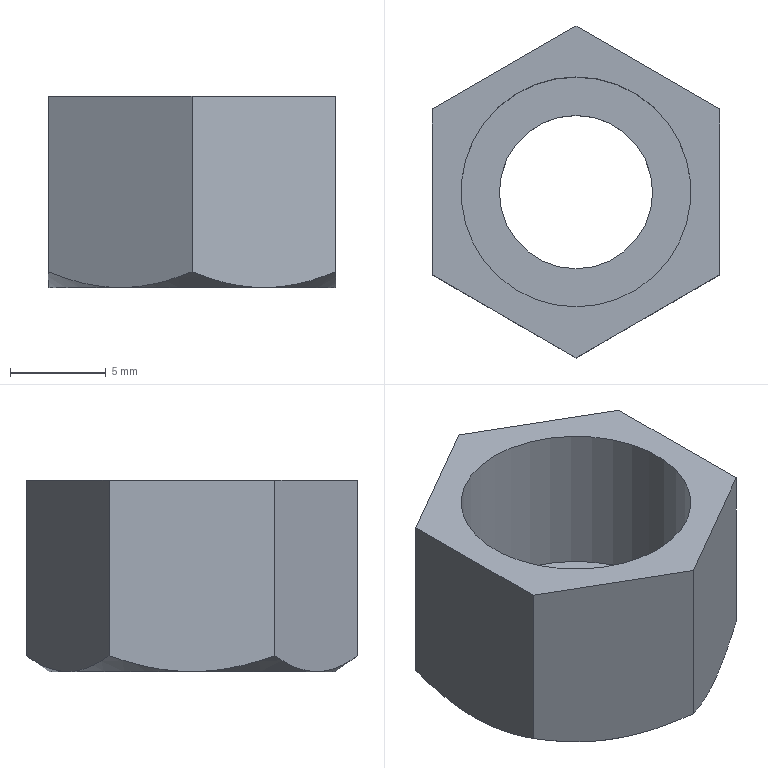Part | STEP file | 1-65.5 | 1 solid | 12 faces | box 15 x 17.321 x 10 mm | volume 938.524 mm3 | plane 9 | cylinder 2 | cone 1 | commonest cylinder face diameters 8 x1 12 x1
STEP:
#1=CARTESIAN_POINT('',(0.,0.,0.));
#2=DIRECTION('',(0.,0.,1.));
#3=DIRECTION('',(1.,0.,0.));
#4=AXIS2_PLACEMENT_3D('',#1,#2,#3);
#5=CARTESIAN_POINT('',(-7.5,-4.33,0.));
#6=VERTEX_POINT('',#5);
#7=CARTESIAN_POINT('',(-7.5,4.33,0.));
#8=VERTEX_POINT('',#7);
#9=CARTESIAN_POINT('',(-7.5,-4.33,0.));
#10=DIRECTION('',(0.,1.,0.));
#11=VECTOR('',#10,1.);
#12=LINE('',#9,#11);
#13=CARTESIAN_POINT('',(1.16,0.,0.));
#14=DIRECTION('',(0.,0.,-1.));
#15=DIRECTION('',(1.,0.,0.));
#16=AXIS2_PLACEMENT_3D('',#13,#14,#15);
#17=PLANE('',#16);
#18=CARTESIAN_POINT('',(-8.66,4.33));
#19=DIRECTION('',(0.,-1.));
#20=VECTOR('',#19,1.);
#21=LINE('',#18,#20);
#22=(GEOMETRIC_REPRESENTATION_CONTEXT(2)PARAMETRIC_REPRESENTATION_CONTEXT()REPRESENTATION_CONTEXT('',''));
#23=DEFINITIONAL_REPRESENTATION('',(#21),#22);
#24=PCURVE('',#17,#23);
#25=CARTESIAN_POINT('',(-7.5,0.,-5.));
#26=DIRECTION('',(-1.,0.,0.));
#27=DIRECTION('',(0.,1.,0.));
#28=AXIS2_PLACEMENT_3D('',#25,#26,#27);
#29=PLANE('',#28);
#30=CARTESIAN_POINT('',(-4.33,-5.));
#31=DIRECTION('',(1.,0.));
#32=VECTOR('',#31,1.);
#33=LINE('',#30,#32);
#34=(GEOMETRIC_REPRESENTATION_CONTEXT(2)PARAMETRIC_REPRESENTATION_CONTEXT()REPRESENTATION_CONTEXT('',''));
#35=DEFINITIONAL_REPRESENTATION('',(#33),#34);
#36=PCURVE('',#29,#35);
#37=SURFACE_CURVE('',#12,(#24,#36),.PCURVE_S1.);
#38=EDGE_CURVE('',#6,#8,#37,.T.);
#39=ORIENTED_EDGE('',*,*,#38,.T.);
#40=CARTESIAN_POINT('',(0.,8.66,0.));
#41=VERTEX_POINT('',#40);
#42=CARTESIAN_POINT('',(-7.5,4.33,0.));
#43=DIRECTION('',(0.866,0.5,0.));
#44=VECTOR('',#43,1.);
#45=LINE('',#42,#44);
#46=CARTESIAN_POINT('',(-8.66,-4.33));
#47=DIRECTION('',(0.866,-0.5));
#48=VECTOR('',#47,1.);
#49=LINE('',#46,#48);
#50=(GEOMETRIC_REPRESENTATION_CONTEXT(2)PARAMETRIC_REPRESENTATION_CONTEXT()REPRESENTATION_CONTEXT('',''));
#51=DEFINITIONAL_REPRESENTATION('',(#49),#50);
#52=PCURVE('',#17,#51);
#53=CARTESIAN_POINT('',(-3.75,6.495,-5.));
#54=DIRECTION('',(-0.5,0.866,0.));
#55=DIRECTION('',(0.866,0.5,0.));
#56=AXIS2_PLACEMENT_3D('',#53,#54,#55);
#57=PLANE('',#56);
#58=CARTESIAN_POINT('',(-4.33,-5.));
#59=DIRECTION('',(1.,0.));
#60=VECTOR('',#59,1.);
#61=LINE('',#58,#60);
#62=(GEOMETRIC_REPRESENTATION_CONTEXT(2)PARAMETRIC_REPRESENTATION_CONTEXT()REPRESENTATION_CONTEXT('',''));
#63=DEFINITIONAL_REPRESENTATION('',(#61),#62);
#64=PCURVE('',#57,#63);
#65=SURFACE_CURVE('',#45,(#52,#64),.PCURVE_S1.);
#66=EDGE_CURVE('',#8,#41,#65,.T.);
#67=ORIENTED_EDGE('',*,*,#66,.T.);
#68=CARTESIAN_POINT('',(7.5,4.33,0.));
#69=VERTEX_POINT('',#68);
#70=CARTESIAN_POINT('',(0.,8.66,0.));
#71=DIRECTION('',(0.866,-0.5,0.));
#72=VECTOR('',#71,1.);
#73=LINE('',#70,#72);
#74=CARTESIAN_POINT('',(-1.16,-8.66));
#75=DIRECTION('',(0.866,0.5));
#76=VECTOR('',#75,1.);
#77=LINE('',#74,#76);
#78=(GEOMETRIC_REPRESENTATION_CONTEXT(2)PARAMETRIC_REPRESENTATION_CONTEXT()REPRESENTATION_CONTEXT('',''));
#79=DEFINITIONAL_REPRESENTATION('',(#77),#78);
#80=PCURVE('',#17,#79);
#81=CARTESIAN_POINT('',(3.75,6.495,-5.));
#82=DIRECTION('',(0.5,0.866,0.));
#83=DIRECTION('',(0.866,-0.5,0.));
#84=AXIS2_PLACEMENT_3D('',#81,#82,#83);
#85=PLANE('',#84);
#86=CARTESIAN_POINT('',(-4.33,-5.));
#87=DIRECTION('',(1.,0.));
#88=VECTOR('',#87,1.);
#89=LINE('',#86,#88);
#90=(GEOMETRIC_REPRESENTATION_CONTEXT(2)PARAMETRIC_REPRESENTATION_CONTEXT()REPRESENTATION_CONTEXT('',''));
#91=DEFINITIONAL_REPRESENTATION('',(#89),#90);
#92=PCURVE('',#85,#91);
#93=SURFACE_CURVE('',#73,(#80,#92),.PCURVE_S1.);
#94=EDGE_CURVE('',#41,#69,#93,.T.);
#95=ORIENTED_EDGE('',*,*,#94,.T.);
#96=CARTESIAN_POINT('',(7.5,-4.33,0.));
#97=VERTEX_POINT('',#96);
#98=CARTESIAN_POINT('',(7.5,4.33,0.));
#99=DIRECTION('',(0.,-1.,0.));
#100=VECTOR('',#99,1.);
#101=LINE('',#98,#100);
#102=CARTESIAN_POINT('',(6.34,-4.33));
#103=DIRECTION('',(0.,1.));
#104=VECTOR('',#103,1.);
#105=LINE('',#102,#104);
#106=(GEOMETRIC_REPRESENTATION_CONTEXT(2)PARAMETRIC_REPRESENTATION_CONTEXT()REPRESENTATION_CONTEXT('',''));
#107=DEFINITIONAL_REPRESENTATION('',(#105),#106);
#108=PCURVE('',#17,#107);
#109=CARTESIAN_POINT('',(7.5,0.,-5.));
#110=DIRECTION('',(1.,0.,0.));
#111=DIRECTION('',(0.,-1.,0.));
#112=AXIS2_PLACEMENT_3D('',#109,#110,#111);
#113=PLANE('',#112);
#114=CARTESIAN_POINT('',(-4.33,-5.));
#115=DIRECTION('',(1.,0.));
#116=VECTOR('',#115,1.);
#117=LINE('',#114,#116);
#118=(GEOMETRIC_REPRESENTATION_CONTEXT(2)PARAMETRIC_REPRESENTATION_CONTEXT()REPRESENTATION_CONTEXT('',''));
#119=DEFINITIONAL_REPRESENTATION('',(#117),#118);
#120=PCURVE('',#113,#119);
#121=SURFACE_CURVE('',#101,(#108,#120),.PCURVE_S1.);
#122=EDGE_CURVE('',#69,#97,#121,.T.);
#123=ORIENTED_EDGE('',*,*,#122,.T.);
#124=CARTESIAN_POINT('',(0.,-8.66,0.));
#125=VERTEX_POINT('',#124);
#126=CARTESIAN_POINT('',(7.5,-4.33,0.));
#127=DIRECTION('',(-0.866,-0.5,0.));
#128=VECTOR('',#127,1.);
#129=LINE('',#126,#128);
#130=CARTESIAN_POINT('',(6.34,4.33));
#131=DIRECTION('',(-0.866,0.5));
#132=VECTOR('',#131,1.);
#133=LINE('',#130,#132);
#134=(GEOMETRIC_REPRESENTATION_CONTEXT(2)PARAMETRIC_REPRESENTATION_CONTEXT()REPRESENTATION_CONTEXT('',''));
#135=DEFINITIONAL_REPRESENTATION('',(#133),#134);
#136=PCURVE('',#17,#135);
#137=CARTESIAN_POINT('',(3.75,-6.495,-5.));
#138=DIRECTION('',(0.5,-0.866,0.));
#139=DIRECTION('',(-0.866,-0.5,0.));
#140=AXIS2_PLACEMENT_3D('',#137,#138,#139);
#141=PLANE('',#140);
#142=CARTESIAN_POINT('',(-4.33,-5.));
#143=DIRECTION('',(1.,0.));
#144=VECTOR('',#143,1.);
#145=LINE('',#142,#144);
#146=(GEOMETRIC_REPRESENTATION_CONTEXT(2)PARAMETRIC_REPRESENTATION_CONTEXT()REPRESENTATION_CONTEXT('',''));
#147=DEFINITIONAL_REPRESENTATION('',(#145),#146);
#148=PCURVE('',#141,#147);
#149=SURFACE_CURVE('',#129,(#136,#148),.PCURVE_S1.);
#150=EDGE_CURVE('',#97,#125,#149,.T.);
#151=ORIENTED_EDGE('',*,*,#150,.T.);
#152=CARTESIAN_POINT('',(0.,-8.66,0.));
#153=DIRECTION('',(-0.866,0.5,0.));
#154=VECTOR('',#153,1.);
#155=LINE('',#152,#154);
#156=CARTESIAN_POINT('',(-1.16,8.66));
#157=DIRECTION('',(-0.866,-0.5));
#158=VECTOR('',#157,1.);
#159=LINE('',#156,#158);
#160=(GEOMETRIC_REPRESENTATION_CONTEXT(2)PARAMETRIC_REPRESENTATION_CONTEXT()REPRESENTATION_CONTEXT('',''));
#161=DEFINITIONAL_REPRESENTATION('',(#159),#160);
#162=PCURVE('',#17,#161);
#163=CARTESIAN_POINT('',(-3.75,-6.495,-5.));
#164=DIRECTION('',(-0.5,-0.866,0.));
#165=DIRECTION('',(-0.866,0.5,0.));
#166=AXIS2_PLACEMENT_3D('',#163,#164,#165);
#167=PLANE('',#166);
#168=CARTESIAN_POINT('',(-4.33,-5.));
#169=DIRECTION('',(1.,0.));
#170=VECTOR('',#169,1.);
#171=LINE('',#168,#170);
#172=(GEOMETRIC_REPRESENTATION_CONTEXT(2)PARAMETRIC_REPRESENTATION_CONTEXT()REPRESENTATION_CONTEXT('',''));
#173=DEFINITIONAL_REPRESENTATION('',(#171),#172);
#174=PCURVE('',#167,#173);
#175=SURFACE_CURVE('',#155,(#162,#174),.PCURVE_S1.);
#176=EDGE_CURVE('',#125,#6,#175,.T.);
#177=ORIENTED_EDGE('',*,*,#176,.T.);
#178=EDGE_LOOP('',(#39,#67,#95,#123,#151,#177));
#179=FACE_BOUND('',#178,.F.);
#180=CARTESIAN_POINT('',(0.,6.,0.));
#181=VERTEX_POINT('',#180);
#182=CARTESIAN_POINT('',(0.,0.,0.));
#183=DIRECTION('',(0.,0.,1.));
#184=DIRECTION('',(0.,1.,0.));
#185=AXIS2_PLACEMENT_3D('',#182,#183,#184);
#186=CIRCLE('',#185,6.);
#187=CARTESIAN_POINT('',(-1.16,-6.));
#188=CARTESIAN_POINT('',(-11.553,-6.));
#189=CARTESIAN_POINT('',(-6.356,3.));
#190=CARTESIAN_POINT('',(-1.16,12.));
#191=CARTESIAN_POINT('',(4.036,3.));
#192=CARTESIAN_POINT('',(9.232,-6.));
#193=CARTESIAN_POINT('',(-1.16,-6.));
#194=(BOUNDED_CURVE()B_SPLINE_CURVE(2,(#187,#188,#189,#190,#191,#192,#193),.UNSPECIFIED.,.T.,.F.)B_SPLINE_CURVE_WITH_KNOTS((1,2,2,2,2,1),(-2.094,0.,2.094,4.189,6.283,8.378),.UNSPECIFIED.)CURVE()GEOMETRIC_REPRESENTATION_ITEM()RATIONAL_B_SPLINE_CURVE((1.,0.5,1.,0.5,1.,0.5,1.))REPRESENTATION_ITEM(''));
#195=(GEOMETRIC_REPRESENTATION_CONTEXT(2)PARAMETRIC_REPRESENTATION_CONTEXT()REPRESENTATION_CONTEXT('',''));
#196=DEFINITIONAL_REPRESENTATION('',(#194),#195);
#197=PCURVE('',#17,#196);
#198=CARTESIAN_POINT('',(0.,0.,0.));
#199=DIRECTION('',(0.,0.,-1.));
#200=DIRECTION('',(0.,1.,0.));
#201=AXIS2_PLACEMENT_3D('',#198,#199,#200);
#202=CYLINDRICAL_SURFACE('',#201,6.);
#203=CARTESIAN_POINT('',(6.283,0.));
#204=DIRECTION('',(-1.,0.));
#205=VECTOR('',#204,1.);
#206=LINE('',#203,#205);
#207=(GEOMETRIC_REPRESENTATION_CONTEXT(2)PARAMETRIC_REPRESENTATION_CONTEXT()REPRESENTATION_CONTEXT('',''));
#208=DEFINITIONAL_REPRESENTATION('',(#206),#207);
#209=PCURVE('',#202,#208);
#210=SURFACE_CURVE('',#186,(#197,#209),.PCURVE_S1.);
#211=EDGE_CURVE('',#181,#181,#210,.T.);
#212=ORIENTED_EDGE('',*,*,#211,.T.);
#213=EDGE_LOOP('',(#212));
#214=FACE_BOUND('',#213,.F.);
#215=ADVANCED_FACE('',(#179,#214),#17,.F.);
#216=CARTESIAN_POINT('',(0.,6.,-8.));
#217=VERTEX_POINT('',#216);
#218=CARTESIAN_POINT('',(0.,6.,0.));
#219=DIRECTION('',(0.,0.,-1.));
#220=VECTOR('',#219,1.);
#221=LINE('',#218,#220);
#222=CARTESIAN_POINT('',(6.283,0.));
#223=DIRECTION('',(0.,1.));
#224=VECTOR('',#223,1.);
#225=LINE('',#222,#224);
#226=(GEOMETRIC_REPRESENTATION_CONTEXT(2)PARAMETRIC_REPRESENTATION_CONTEXT()REPRESENTATION_CONTEXT('',''));
#227=DEFINITIONAL_REPRESENTATION('',(#225),#226);
#228=PCURVE('',#202,#227);
#229=CARTESIAN_POINT('',(0.,0.));
#230=DIRECTION('',(0.,1.));
#231=VECTOR('',#230,1.);
#232=LINE('',#229,#231);
#233=(GEOMETRIC_REPRESENTATION_CONTEXT(2)PARAMETRIC_REPRESENTATION_CONTEXT()REPRESENTATION_CONTEXT('',''));
#234=DEFINITIONAL_REPRESENTATION('',(#232),#233);
#235=PCURVE('',#202,#234);
#236=SEAM_CURVE('',#221,(#228,#235),.PCURVE_S1.);
#237=EDGE_CURVE('',#181,#217,#236,.T.);
#238=ORIENTED_EDGE('',*,*,#237,.T.);
#239=CARTESIAN_POINT('',(0.,0.,-8.));
#240=DIRECTION('',(0.,0.,1.));
#241=DIRECTION('',(0.,1.,0.));
#242=AXIS2_PLACEMENT_3D('',#239,#240,#241);
#243=CIRCLE('',#242,6.);
#244=CARTESIAN_POINT('',(6.283,8.));
#245=DIRECTION('',(-1.,0.));
#246=VECTOR('',#245,1.);
#247=LINE('',#244,#246);
#248=(GEOMETRIC_REPRESENTATION_CONTEXT(2)PARAMETRIC_REPRESENTATION_CONTEXT()REPRESENTATION_CONTEXT('',''));
#249=DEFINITIONAL_REPRESENTATION('',(#247),#248);
#250=PCURVE('',#202,#249);
#251=CARTESIAN_POINT('',(0.,-1.608,-8.));
#252=DIRECTION('',(0.,0.,1.));
#253=DIRECTION('',(1.,0.,0.));
#254=AXIS2_PLACEMENT_3D('',#251,#252,#253);
#255=PLANE('',#254);
#256=CARTESIAN_POINT('',(0.,1.608));
#257=DIRECTION('',(0.,1.));
#258=AXIS2_PLACEMENT_2D('',#256,#257);
#259=CIRCLE('',#258,6.);
#260=(GEOMETRIC_REPRESENTATION_CONTEXT(2)PARAMETRIC_REPRESENTATION_CONTEXT()REPRESENTATION_CONTEXT('',''));
#261=DEFINITIONAL_REPRESENTATION('',(#259),#260);
#262=PCURVE('',#255,#261);
#263=SURFACE_CURVE('',#243,(#250,#262),.PCURVE_S1.);
#264=EDGE_CURVE('',#217,#217,#263,.T.);
#265=ORIENTED_EDGE('',*,*,#264,.T.);
#266=ORIENTED_EDGE('',*,*,#237,.F.);
#267=ORIENTED_EDGE('',*,*,#211,.F.);
#268=EDGE_LOOP('',(#238,#265,#266,#267));
#269=FACE_BOUND('',#268,.F.);
#270=ADVANCED_FACE('',(#269),#202,.F.);
#271=ORIENTED_EDGE('',*,*,#264,.T.);
#272=EDGE_LOOP('',(#271));
#273=FACE_BOUND('',#272,.T.);
#274=CARTESIAN_POINT('',(0.,4.,-8.));
#275=VERTEX_POINT('',#274);
#276=CARTESIAN_POINT('',(0.,0.,-8.));
#277=DIRECTION('',(0.,0.,1.));
#278=DIRECTION('',(0.,1.,0.));
#279=AXIS2_PLACEMENT_3D('',#276,#277,#278);
#280=CIRCLE('',#279,4.);
#281=CARTESIAN_POINT('',(0.,1.608));
#282=DIRECTION('',(0.,1.));
#283=AXIS2_PLACEMENT_2D('',#281,#282);
#284=CIRCLE('',#283,4.);
#285=(GEOMETRIC_REPRESENTATION_CONTEXT(2)PARAMETRIC_REPRESENTATION_CONTEXT()REPRESENTATION_CONTEXT('',''));
#286=DEFINITIONAL_REPRESENTATION('',(#284),#285);
#287=PCURVE('',#255,#286);
#288=CARTESIAN_POINT('',(0.,0.,0.));
#289=DIRECTION('',(0.,0.,-1.));
#290=DIRECTION('',(0.,1.,0.));
#291=AXIS2_PLACEMENT_3D('',#288,#289,#290);
#292=CYLINDRICAL_SURFACE('',#291,4.);
#293=CARTESIAN_POINT('',(6.283,8.));
#294=DIRECTION('',(-1.,0.));
#295=VECTOR('',#294,1.);
#296=LINE('',#293,#295);
#297=(GEOMETRIC_REPRESENTATION_CONTEXT(2)PARAMETRIC_REPRESENTATION_CONTEXT()REPRESENTATION_CONTEXT('',''));
#298=DEFINITIONAL_REPRESENTATION('',(#296),#297);
#299=PCURVE('',#292,#298);
#300=SURFACE_CURVE('',#280,(#287,#299),.PCURVE_S1.);
#301=EDGE_CURVE('',#275,#275,#300,.T.);
#302=ORIENTED_EDGE('',*,*,#301,.F.);
#303=EDGE_LOOP('',(#302));
#304=FACE_BOUND('',#303,.T.);
#305=ADVANCED_FACE('',(#273,#304),#255,.T.);
#306=CARTESIAN_POINT('',(0.,4.,-10.));
#307=VERTEX_POINT('',#306);
#308=CARTESIAN_POINT('',(0.,4.,-8.));
#309=DIRECTION('',(0.,0.,-1.));
#310=VECTOR('',#309,1.);
#311=LINE('',#308,#310);
#312=CARTESIAN_POINT('',(0.,8.));
#313=DIRECTION('',(0.,1.));
#314=VECTOR('',#313,1.);
#315=LINE('',#312,#314);
#316=(GEOMETRIC_REPRESENTATION_CONTEXT(2)PARAMETRIC_REPRESENTATION_CONTEXT()REPRESENTATION_CONTEXT('',''));
#317=DEFINITIONAL_REPRESENTATION('',(#315),#316);
#318=PCURVE('',#292,#317);
#319=CARTESIAN_POINT('',(6.283,8.));
#320=DIRECTION('',(0.,1.));
#321=VECTOR('',#320,1.);
#322=LINE('',#319,#321);
#323=(GEOMETRIC_REPRESENTATION_CONTEXT(2)PARAMETRIC_REPRESENTATION_CONTEXT()REPRESENTATION_CONTEXT('',''));
#324=DEFINITIONAL_REPRESENTATION('',(#322),#323);
#325=PCURVE('',#292,#324);
#326=SEAM_CURVE('',#311,(#318,#325),.PCURVE_S1.);
#327=EDGE_CURVE('',#275,#307,#326,.T.);
#328=ORIENTED_EDGE('',*,*,#327,.F.);
#329=ORIENTED_EDGE('',*,*,#301,.F.);
#330=ORIENTED_EDGE('',*,*,#327,.T.);
#331=CARTESIAN_POINT('',(0.,0.,-10.));
#332=DIRECTION('',(0.,0.,1.));
#333=DIRECTION('',(0.,1.,0.));
#334=AXIS2_PLACEMENT_3D('',#331,#332,#333);
#335=CIRCLE('',#334,4.);
#336=CARTESIAN_POINT('',(6.283,10.));
#337=DIRECTION('',(-1.,0.));
#338=VECTOR('',#337,1.);
#339=LINE('',#336,#338);
#340=(GEOMETRIC_REPRESENTATION_CONTEXT(2)PARAMETRIC_REPRESENTATION_CONTEXT()REPRESENTATION_CONTEXT('',''));
#341=DEFINITIONAL_REPRESENTATION('',(#339),#340);
#342=PCURVE('',#292,#341);
#343=CARTESIAN_POINT('',(1.16,0.,-10.));
#344=DIRECTION('',(0.,0.,-1.));
#345=DIRECTION('',(1.,0.,0.));
#346=AXIS2_PLACEMENT_3D('',#343,#344,#345);
#347=PLANE('',#346);
#348=CARTESIAN_POINT('',(-1.16,-4.));
#349=CARTESIAN_POINT('',(-8.088,-4.));
#350=CARTESIAN_POINT('',(-4.624,2.));
#351=CARTESIAN_POINT('',(-1.16,8.));
#352=CARTESIAN_POINT('',(2.304,2.));
#353=CARTESIAN_POINT('',(5.768,-4.));
#354=CARTESIAN_POINT('',(-1.16,-4.));
#355=(BOUNDED_CURVE()B_SPLINE_CURVE(2,(#348,#349,#350,#351,#352,#353,#354),.UNSPECIFIED.,.T.,.F.)B_SPLINE_CURVE_WITH_KNOTS((1,2,2,2,2,1),(-2.094,0.,2.094,4.189,6.283,8.378),.UNSPECIFIED.)CURVE()GEOMETRIC_REPRESENTATION_ITEM()RATIONAL_B_SPLINE_CURVE((1.,0.5,1.,0.5,1.,0.5,1.))REPRESENTATION_ITEM(''));
#356=(GEOMETRIC_REPRESENTATION_CONTEXT(2)PARAMETRIC_REPRESENTATION_CONTEXT()REPRESENTATION_CONTEXT('',''));
#357=DEFINITIONAL_REPRESENTATION('',(#355),#356);
#358=PCURVE('',#347,#357);
#359=SURFACE_CURVE('',#335,(#342,#358),.PCURVE_S1.);
#360=EDGE_CURVE('',#307,#307,#359,.T.);
#361=ORIENTED_EDGE('',*,*,#360,.T.);
#362=EDGE_LOOP('',(#328,#329,#330,#361));
#363=FACE_BOUND('',#362,.F.);
#364=ADVANCED_FACE('',(#363),#292,.F.);
#365=ORIENTED_EDGE('',*,*,#38,.T.);
#366=CARTESIAN_POINT('',(-7.5,4.33,-9.163));
#367=VERTEX_POINT('',#366);
#368=CARTESIAN_POINT('',(-7.5,4.33,0.));
#369=DIRECTION('',(0.,0.,-1.));
#370=VECTOR('',#369,1.);
#371=LINE('',#368,#370);
#372=CARTESIAN_POINT('',(4.33,-5.));
#373=DIRECTION('',(0.,1.));
#374=VECTOR('',#373,1.);
#375=LINE('',#372,#374);
#376=(GEOMETRIC_REPRESENTATION_CONTEXT(2)PARAMETRIC_REPRESENTATION_CONTEXT()REPRESENTATION_CONTEXT('',''));
#377=DEFINITIONAL_REPRESENTATION('',(#375),#376);
#378=PCURVE('',#29,#377);
#379=CARTESIAN_POINT('',(-4.33,-5.));
#380=DIRECTION('',(0.,1.));
#381=VECTOR('',#380,1.);
#382=LINE('',#379,#381);
#383=(GEOMETRIC_REPRESENTATION_CONTEXT(2)PARAMETRIC_REPRESENTATION_CONTEXT()REPRESENTATION_CONTEXT('',''));
#384=DEFINITIONAL_REPRESENTATION('',(#382),#383);
#385=PCURVE('',#57,#384);
#386=SURFACE_CURVE('',#371,(#378,#385),.PCURVE_S1.);
#387=EDGE_CURVE('',#8,#367,#386,.T.);
#388=ORIENTED_EDGE('',*,*,#387,.T.);
#389=CARTESIAN_POINT('',(-7.5,-4.33,-9.163));
#390=VERTEX_POINT('',#389);
#391=CARTESIAN_POINT('',(-7.5,-4.33,-9.163));
#392=CARTESIAN_POINT('',(-7.5,0.,-10.704));
#393=CARTESIAN_POINT('',(-7.5,4.33,-9.163));
#394=(BOUNDED_CURVE()B_SPLINE_CURVE(2,(#391,#392,#393),.UNSPECIFIED.,.F.,.F.)B_SPLINE_CURVE_WITH_KNOTS((3,3),(0.,1.),.PIECEWISE_BEZIER_KNOTS.)CURVE()GEOMETRIC_REPRESENTATION_ITEM()RATIONAL_B_SPLINE_CURVE((1.425,1.645,1.425))REPRESENTATION_ITEM(''));
#395=CARTESIAN_POINT('',(-4.33,4.163));
#396=CARTESIAN_POINT('',(0.,5.704));
#397=CARTESIAN_POINT('',(4.33,4.163));
#398=(BOUNDED_CURVE()B_SPLINE_CURVE(2,(#395,#396,#397),.UNSPECIFIED.,.F.,.F.)B_SPLINE_CURVE_WITH_KNOTS((3,3),(0.,1.),.PIECEWISE_BEZIER_KNOTS.)CURVE()GEOMETRIC_REPRESENTATION_ITEM()RATIONAL_B_SPLINE_CURVE((1.425,1.645,1.425))REPRESENTATION_ITEM(''));
#399=(GEOMETRIC_REPRESENTATION_CONTEXT(2)PARAMETRIC_REPRESENTATION_CONTEXT()REPRESENTATION_CONTEXT('',''));
#400=DEFINITIONAL_REPRESENTATION('',(#398),#399);
#401=PCURVE('',#29,#400);
#402=CARTESIAN_POINT('',(0.,0.,-10.));
#403=DIRECTION('',(0.,0.,1.));
#404=DIRECTION('',(1.,0.,0.));
#405=AXIS2_PLACEMENT_3D('',#402,#403,#404);
#406=CONICAL_SURFACE('',#405,7.484,0.9523);
#407=CARTESIAN_POINT('',(3.665,0.8369));
#408=CARTESIAN_POINT('',(3.65,0.783));
#409=CARTESIAN_POINT('',(3.62,0.6816));
#410=CARTESIAN_POINT('',(3.573,0.5474));
#411=CARTESIAN_POINT('',(3.527,0.4299));
#412=CARTESIAN_POINT('',(3.479,0.3283));
#413=CARTESIAN_POINT('',(3.432,0.2418));
#414=CARTESIAN_POINT('',(3.384,0.1696));
#415=CARTESIAN_POINT('',(3.336,0.1113));
#416=CARTESIAN_POINT('',(3.288,0.06633));
#417=CARTESIAN_POINT('',(3.239,0.03445));
#418=CARTESIAN_POINT('',(3.19,0.01541));
#419=CARTESIAN_POINT('',(3.142,0.009081));
#420=CARTESIAN_POINT('',(3.093,0.01541));
#421=CARTESIAN_POINT('',(3.044,0.03445));
#422=CARTESIAN_POINT('',(2.996,0.06633));
#423=CARTESIAN_POINT('',(2.947,0.1113));
#424=CARTESIAN_POINT('',(2.899,0.1696));
#425=CARTESIAN_POINT('',(2.851,0.2418));
#426=CARTESIAN_POINT('',(2.804,0.3283));
#427=CARTESIAN_POINT('',(2.757,0.4299));
#428=CARTESIAN_POINT('',(2.71,0.5474));
#429=CARTESIAN_POINT('',(2.664,0.6816));
#430=CARTESIAN_POINT('',(2.633,0.783));
#431=CARTESIAN_POINT('',(2.618,0.8369));
#432=B_SPLINE_CURVE_WITH_KNOTS('',3,(#407,#408,#409,#410,#411,#412,#413,#414,#415,#416,#417,#418,#419,#420,#421,#422,#423,#424,#425,#426,#427,#428,#429,#430,#431),.UNSPECIFIED.,.F.,.F.,(4,1,1,1,1,1,1,1,1,1,1,1,1,1,1,1,1,1,1,1,1,1,4),(0.,0.04545,0.09091,0.1364,0.1818,0.2273,0.2727,0.3182,0.3636,0.4091,0.4545,0.5,0.5455,0.5909,0.6364,0.6818,0.7273,0.7727,0.8182,0.8636,0.9091,0.9545,1.),.QUASI_UNIFORM_KNOTS.);
#433=(GEOMETRIC_REPRESENTATION_CONTEXT(2)PARAMETRIC_REPRESENTATION_CONTEXT()REPRESENTATION_CONTEXT('',''));
#434=DEFINITIONAL_REPRESENTATION('',(#432),#433);
#435=PCURVE('',#406,#434);
#436=SURFACE_CURVE('',#394,(#401,#435),.PCURVE_S1.);
#437=EDGE_CURVE('',#390,#367,#436,.T.);
#438=ORIENTED_EDGE('',*,*,#437,.F.);
#439=CARTESIAN_POINT('',(-7.5,-4.33,0.));
#440=DIRECTION('',(0.,0.,-1.));
#441=VECTOR('',#440,1.);
#442=LINE('',#439,#441);
#443=CARTESIAN_POINT('',(-4.33,-5.));
#444=DIRECTION('',(0.,1.));
#445=VECTOR('',#444,1.);
#446=LINE('',#443,#445);
#447=(GEOMETRIC_REPRESENTATION_CONTEXT(2)PARAMETRIC_REPRESENTATION_CONTEXT()REPRESENTATION_CONTEXT('',''));
#448=DEFINITIONAL_REPRESENTATION('',(#446),#447);
#449=PCURVE('',#29,#448);
#450=CARTESIAN_POINT('',(4.33,-5.));
#451=DIRECTION('',(0.,1.));
#452=VECTOR('',#451,1.);
#453=LINE('',#450,#452);
#454=(GEOMETRIC_REPRESENTATION_CONTEXT(2)PARAMETRIC_REPRESENTATION_CONTEXT()REPRESENTATION_CONTEXT('',''));
#455=DEFINITIONAL_REPRESENTATION('',(#453),#454);
#456=PCURVE('',#167,#455);
#457=SURFACE_CURVE('',#442,(#449,#456),.PCURVE_S1.);
#458=EDGE_CURVE('',#6,#390,#457,.T.);
#459=ORIENTED_EDGE('',*,*,#458,.F.);
#460=EDGE_LOOP('',(#365,#388,#438,#459));
#461=FACE_BOUND('',#460,.T.);
#462=ADVANCED_FACE('',(#461),#29,.T.);
#463=ORIENTED_EDGE('',*,*,#66,.T.);
#464=CARTESIAN_POINT('',(0.,8.66,-9.163));
#465=VERTEX_POINT('',#464);
#466=CARTESIAN_POINT('',(0.,8.66,0.));
#467=DIRECTION('',(0.,0.,-1.));
#468=VECTOR('',#467,1.);
#469=LINE('',#466,#468);
#470=CARTESIAN_POINT('',(4.33,-5.));
#471=DIRECTION('',(0.,1.));
#472=VECTOR('',#471,1.);
#473=LINE('',#470,#472);
#474=(GEOMETRIC_REPRESENTATION_CONTEXT(2)PARAMETRIC_REPRESENTATION_CONTEXT()REPRESENTATION_CONTEXT('',''));
#475=DEFINITIONAL_REPRESENTATION('',(#473),#474);
#476=PCURVE('',#57,#475);
#477=CARTESIAN_POINT('',(-4.33,-5.));
#478=DIRECTION('',(0.,1.));
#479=VECTOR('',#478,1.);
#480=LINE('',#477,#479);
#481=(GEOMETRIC_REPRESENTATION_CONTEXT(2)PARAMETRIC_REPRESENTATION_CONTEXT()REPRESENTATION_CONTEXT('',''));
#482=DEFINITIONAL_REPRESENTATION('',(#480),#481);
#483=PCURVE('',#85,#482);
#484=SURFACE_CURVE('',#469,(#476,#483),.PCURVE_S1.);
#485=EDGE_CURVE('',#41,#465,#484,.T.);
#486=ORIENTED_EDGE('',*,*,#485,.T.);
#487=CARTESIAN_POINT('',(-7.5,4.33,-9.163));
#488=CARTESIAN_POINT('',(-3.75,6.495,-10.704));
#489=CARTESIAN_POINT('',(0.,8.66,-9.163));
#490=(BOUNDED_CURVE()B_SPLINE_CURVE(2,(#487,#488,#489),.UNSPECIFIED.,.F.,.F.)B_SPLINE_CURVE_WITH_KNOTS((3,3),(0.,1.),.PIECEWISE_BEZIER_KNOTS.)CURVE()GEOMETRIC_REPRESENTATION_ITEM()RATIONAL_B_SPLINE_CURVE((1.425,1.645,1.425))REPRESENTATION_ITEM(''));
#491=CARTESIAN_POINT('',(-4.33,4.163));
#492=CARTESIAN_POINT('',(0.,5.704));
#493=CARTESIAN_POINT('',(4.33,4.163));
#494=(BOUNDED_CURVE()B_SPLINE_CURVE(2,(#491,#492,#493),.UNSPECIFIED.,.F.,.F.)B_SPLINE_CURVE_WITH_KNOTS((3,3),(0.,1.),.PIECEWISE_BEZIER_KNOTS.)CURVE()GEOMETRIC_REPRESENTATION_ITEM()RATIONAL_B_SPLINE_CURVE((1.425,1.645,1.425))REPRESENTATION_ITEM(''));
#495=(GEOMETRIC_REPRESENTATION_CONTEXT(2)PARAMETRIC_REPRESENTATION_CONTEXT()REPRESENTATION_CONTEXT('',''));
#496=DEFINITIONAL_REPRESENTATION('',(#494),#495);
#497=PCURVE('',#57,#496);
#498=CARTESIAN_POINT('',(2.618,0.8369));
#499=CARTESIAN_POINT('',(2.603,0.783));
#500=CARTESIAN_POINT('',(2.572,0.6816));
#501=CARTESIAN_POINT('',(2.526,0.5474));
#502=CARTESIAN_POINT('',(2.479,0.4299));
#503=CARTESIAN_POINT('',(2.432,0.3283));
#504=CARTESIAN_POINT('',(2.385,0.2418));
#505=CARTESIAN_POINT('',(2.337,0.1696));
#506=CARTESIAN_POINT('',(2.289,0.1113));
#507=CARTESIAN_POINT('',(2.24,0.06633));
#508=CARTESIAN_POINT('',(2.192,0.03445));
#509=CARTESIAN_POINT('',(2.143,0.01541));
#510=CARTESIAN_POINT('',(2.094,0.009081));
#511=CARTESIAN_POINT('',(2.046,0.01541));
#512=CARTESIAN_POINT('',(1.997,0.03445));
#513=CARTESIAN_POINT('',(1.948,0.06633));
#514=CARTESIAN_POINT('',(1.9,0.1113));
#515=CARTESIAN_POINT('',(1.852,0.1696));
#516=CARTESIAN_POINT('',(1.804,0.2418));
#517=CARTESIAN_POINT('',(1.757,0.3283));
#518=CARTESIAN_POINT('',(1.709,0.4299));
#519=CARTESIAN_POINT('',(1.663,0.5474));
#520=CARTESIAN_POINT('',(1.616,0.6816));
#521=CARTESIAN_POINT('',(1.586,0.783));
#522=CARTESIAN_POINT('',(1.571,0.8369));
#523=B_SPLINE_CURVE_WITH_KNOTS('',3,(#498,#499,#500,#501,#502,#503,#504,#505,#506,#507,#508,#509,#510,#511,#512,#513,#514,#515,#516,#517,#518,#519,#520,#521,#522),.UNSPECIFIED.,.F.,.F.,(4,1,1,1,1,1,1,1,1,1,1,1,1,1,1,1,1,1,1,1,1,1,4),(0.,0.04545,0.09091,0.1364,0.1818,0.2273,0.2727,0.3182,0.3636,0.4091,0.4545,0.5,0.5455,0.5909,0.6364,0.6818,0.7273,0.7727,0.8182,0.8636,0.9091,0.9545,1.),.QUASI_UNIFORM_KNOTS.);
#524=(GEOMETRIC_REPRESENTATION_CONTEXT(2)PARAMETRIC_REPRESENTATION_CONTEXT()REPRESENTATION_CONTEXT('',''));
#525=DEFINITIONAL_REPRESENTATION('',(#523),#524);
#526=PCURVE('',#406,#525);
#527=SURFACE_CURVE('',#490,(#497,#526),.PCURVE_S1.);
#528=EDGE_CURVE('',#367,#465,#527,.T.);
#529=ORIENTED_EDGE('',*,*,#528,.F.);
#530=ORIENTED_EDGE('',*,*,#387,.F.);
#531=EDGE_LOOP('',(#463,#486,#529,#530));
#532=FACE_BOUND('',#531,.T.);
#533=ADVANCED_FACE('',(#532),#57,.T.);
#534=ORIENTED_EDGE('',*,*,#94,.T.);
#535=CARTESIAN_POINT('',(7.5,4.33,-9.163));
#536=VERTEX_POINT('',#535);
#537=CARTESIAN_POINT('',(7.5,4.33,0.));
#538=DIRECTION('',(0.,0.,-1.));
#539=VECTOR('',#538,1.);
#540=LINE('',#537,#539);
#541=CARTESIAN_POINT('',(4.33,-5.));
#542=DIRECTION('',(0.,1.));
#543=VECTOR('',#542,1.);
#544=LINE('',#541,#543);
#545=(GEOMETRIC_REPRESENTATION_CONTEXT(2)PARAMETRIC_REPRESENTATION_CONTEXT()REPRESENTATION_CONTEXT('',''));
#546=DEFINITIONAL_REPRESENTATION('',(#544),#545);
#547=PCURVE('',#85,#546);
#548=CARTESIAN_POINT('',(-4.33,-5.));
#549=DIRECTION('',(0.,1.));
#550=VECTOR('',#549,1.);
#551=LINE('',#548,#550);
#552=(GEOMETRIC_REPRESENTATION_CONTEXT(2)PARAMETRIC_REPRESENTATION_CONTEXT()REPRESENTATION_CONTEXT('',''));
#553=DEFINITIONAL_REPRESENTATION('',(#551),#552);
#554=PCURVE('',#113,#553);
#555=SURFACE_CURVE('',#540,(#547,#554),.PCURVE_S1.);
#556=EDGE_CURVE('',#69,#536,#555,.T.);
#557=ORIENTED_EDGE('',*,*,#556,.T.);
#558=CARTESIAN_POINT('',(0.,8.66,-9.163));
#559=CARTESIAN_POINT('',(3.75,6.495,-10.704));
#560=CARTESIAN_POINT('',(7.5,4.33,-9.163));
#561=(BOUNDED_CURVE()B_SPLINE_CURVE(2,(#558,#559,#560),.UNSPECIFIED.,.F.,.F.)B_SPLINE_CURVE_WITH_KNOTS((3,3),(0.,1.),.PIECEWISE_BEZIER_KNOTS.)CURVE()GEOMETRIC_REPRESENTATION_ITEM()RATIONAL_B_SPLINE_CURVE((1.425,1.645,1.425))REPRESENTATION_ITEM(''));
#562=CARTESIAN_POINT('',(-4.33,4.163));
#563=CARTESIAN_POINT('',(0.,5.704));
#564=CARTESIAN_POINT('',(4.33,4.163));
#565=(BOUNDED_CURVE()B_SPLINE_CURVE(2,(#562,#563,#564),.UNSPECIFIED.,.F.,.F.)B_SPLINE_CURVE_WITH_KNOTS((3,3),(0.,1.),.PIECEWISE_BEZIER_KNOTS.)CURVE()GEOMETRIC_REPRESENTATION_ITEM()RATIONAL_B_SPLINE_CURVE((1.425,1.645,1.425))REPRESENTATION_ITEM(''));
#566=(GEOMETRIC_REPRESENTATION_CONTEXT(2)PARAMETRIC_REPRESENTATION_CONTEXT()REPRESENTATION_CONTEXT('',''));
#567=DEFINITIONAL_REPRESENTATION('',(#565),#566);
#568=PCURVE('',#85,#567);
#569=CARTESIAN_POINT('',(1.571,0.8369));
#570=CARTESIAN_POINT('',(1.556,0.783));
#571=CARTESIAN_POINT('',(1.525,0.6816));
#572=CARTESIAN_POINT('',(1.479,0.5474));
#573=CARTESIAN_POINT('',(1.432,0.4299));
#574=CARTESIAN_POINT('',(1.385,0.3283));
#575=CARTESIAN_POINT('',(1.338,0.2418));
#576=CARTESIAN_POINT('',(1.29,0.1696));
#577=CARTESIAN_POINT('',(1.241,0.1113));
#578=CARTESIAN_POINT('',(1.193,0.06633));
#579=CARTESIAN_POINT('',(1.145,0.03445));
#580=CARTESIAN_POINT('',(1.096,0.01541));
#581=CARTESIAN_POINT('',(1.047,0.009081));
#582=CARTESIAN_POINT('',(0.9985,0.01541));
#583=CARTESIAN_POINT('',(0.9498,0.03445));
#584=CARTESIAN_POINT('',(0.9013,0.06633));
#585=CARTESIAN_POINT('',(0.8529,0.1113));
#586=CARTESIAN_POINT('',(0.8048,0.1696));
#587=CARTESIAN_POINT('',(0.7569,0.2418));
#588=CARTESIAN_POINT('',(0.7094,0.3283));
#589=CARTESIAN_POINT('',(0.6622,0.4299));
#590=CARTESIAN_POINT('',(0.6155,0.5474));
#591=CARTESIAN_POINT('',(0.5692,0.6816));
#592=CARTESIAN_POINT('',(0.5388,0.783));
#593=CARTESIAN_POINT('',(0.5236,0.8369));
#594=B_SPLINE_CURVE_WITH_KNOTS('',3,(#569,#570,#571,#572,#573,#574,#575,#576,#577,#578,#579,#580,#581,#582,#583,#584,#585,#586,#587,#588,#589,#590,#591,#592,#593),.UNSPECIFIED.,.F.,.F.,(4,1,1,1,1,1,1,1,1,1,1,1,1,1,1,1,1,1,1,1,1,1,4),(0.,0.04545,0.09091,0.1364,0.1818,0.2273,0.2727,0.3182,0.3636,0.4091,0.4545,0.5,0.5455,0.5909,0.6364,0.6818,0.7273,0.7727,0.8182,0.8636,0.9091,0.9545,1.),.QUASI_UNIFORM_KNOTS.);
#595=(GEOMETRIC_REPRESENTATION_CONTEXT(2)PARAMETRIC_REPRESENTATION_CONTEXT()REPRESENTATION_CONTEXT('',''));
#596=DEFINITIONAL_REPRESENTATION('',(#594),#595);
#597=PCURVE('',#406,#596);
#598=SURFACE_CURVE('',#561,(#568,#597),.PCURVE_S1.);
#599=EDGE_CURVE('',#465,#536,#598,.T.);
#600=ORIENTED_EDGE('',*,*,#599,.F.);
#601=ORIENTED_EDGE('',*,*,#485,.F.);
#602=EDGE_LOOP('',(#534,#557,#600,#601));
#603=FACE_BOUND('',#602,.T.);
#604=ADVANCED_FACE('',(#603),#85,.T.);
#605=ORIENTED_EDGE('',*,*,#122,.T.);
#606=CARTESIAN_POINT('',(7.5,-4.33,-9.163));
#607=VERTEX_POINT('',#606);
#608=CARTESIAN_POINT('',(7.5,-4.33,0.));
#609=DIRECTION('',(0.,0.,-1.));
#610=VECTOR('',#609,1.);
#611=LINE('',#608,#610);
#612=CARTESIAN_POINT('',(4.33,-5.));
#613=DIRECTION('',(0.,1.));
#614=VECTOR('',#613,1.);
#615=LINE('',#612,#614);
#616=(GEOMETRIC_REPRESENTATION_CONTEXT(2)PARAMETRIC_REPRESENTATION_CONTEXT()REPRESENTATION_CONTEXT('',''));
#617=DEFINITIONAL_REPRESENTATION('',(#615),#616);
#618=PCURVE('',#113,#617);
#619=CARTESIAN_POINT('',(-4.33,-5.));
#620=DIRECTION('',(0.,1.));
#621=VECTOR('',#620,1.);
#622=LINE('',#619,#621);
#623=(GEOMETRIC_REPRESENTATION_CONTEXT(2)PARAMETRIC_REPRESENTATION_CONTEXT()REPRESENTATION_CONTEXT('',''));
#624=DEFINITIONAL_REPRESENTATION('',(#622),#623);
#625=PCURVE('',#141,#624);
#626=SURFACE_CURVE('',#611,(#618,#625),.PCURVE_S1.);
#627=EDGE_CURVE('',#97,#607,#626,.T.);
#628=ORIENTED_EDGE('',*,*,#627,.T.);
#629=CARTESIAN_POINT('',(7.5,0.,-9.989));
#630=VERTEX_POINT('',#629);
#631=CARTESIAN_POINT('',(7.5,0.,-9.989));
#632=CARTESIAN_POINT('',(7.5,-2.01,-9.989));
#633=CARTESIAN_POINT('',(7.5,-4.33,-9.163));
#634=(BOUNDED_CURVE()B_SPLINE_CURVE(2,(#631,#632,#633),.UNSPECIFIED.,.F.,.F.)B_SPLINE_CURVE_WITH_KNOTS((3,3),(0.,1.),.PIECEWISE_BEZIER_KNOTS.)CURVE()GEOMETRIC_REPRESENTATION_ITEM()RATIONAL_B_SPLINE_CURVE((1.535,1.535,1.425))REPRESENTATION_ITEM(''));
#635=CARTESIAN_POINT('',(0.,4.989));
#636=CARTESIAN_POINT('',(2.01,4.989));
#637=CARTESIAN_POINT('',(4.33,4.163));
#638=(BOUNDED_CURVE()B_SPLINE_CURVE(2,(#635,#636,#637),.UNSPECIFIED.,.F.,.F.)B_SPLINE_CURVE_WITH_KNOTS((3,3),(0.,1.),.PIECEWISE_BEZIER_KNOTS.)CURVE()GEOMETRIC_REPRESENTATION_ITEM()RATIONAL_B_SPLINE_CURVE((1.535,1.535,1.425))REPRESENTATION_ITEM(''));
#639=(GEOMETRIC_REPRESENTATION_CONTEXT(2)PARAMETRIC_REPRESENTATION_CONTEXT()REPRESENTATION_CONTEXT('',''));
#640=DEFINITIONAL_REPRESENTATION('',(#638),#639);
#641=PCURVE('',#113,#640);
#642=CARTESIAN_POINT('',(6.283,0.01119));
#643=CARTESIAN_POINT('',(6.275,0.01119));
#644=CARTESIAN_POINT('',(6.259,0.01225));
#645=CARTESIAN_POINT('',(6.234,0.017));
#646=CARTESIAN_POINT('',(6.21,0.02493));
#647=CARTESIAN_POINT('',(6.186,0.03605));
#648=CARTESIAN_POINT('',(6.162,0.05039));
#649=CARTESIAN_POINT('',(6.137,0.06796));
#650=CARTESIAN_POINT('',(6.113,0.0888));
#651=CARTESIAN_POINT('',(6.089,0.1129));
#652=CARTESIAN_POINT('',(6.065,0.1404));
#653=CARTESIAN_POINT('',(6.041,0.1713));
#654=CARTESIAN_POINT('',(6.017,0.2057));
#655=CARTESIAN_POINT('',(5.993,0.2436));
#656=CARTESIAN_POINT('',(5.969,0.2851));
#657=CARTESIAN_POINT('',(5.945,0.3302));
#658=CARTESIAN_POINT('',(5.922,0.3791));
#659=CARTESIAN_POINT('',(5.898,0.4319));
#660=CARTESIAN_POINT('',(5.875,0.4886));
#661=CARTESIAN_POINT('',(5.852,0.5495));
#662=CARTESIAN_POINT('',(5.828,0.6145));
#663=CARTESIAN_POINT('',(5.805,0.6838));
#664=CARTESIAN_POINT('',(5.782,0.7576));
#665=CARTESIAN_POINT('',(5.767,0.8099));
#666=CARTESIAN_POINT('',(5.76,0.8369));
#667=B_SPLINE_CURVE_WITH_KNOTS('',3,(#642,#643,#644,#645,#646,#647,#648,#649,#650,#651,#652,#653,#654,#655,#656,#657,#658,#659,#660,#661,#662,#663,#664,#665,#666),.UNSPECIFIED.,.F.,.F.,(4,1,1,1,1,1,1,1,1,1,1,1,1,1,1,1,1,1,1,1,1,1,4),(0.,0.04545,0.09091,0.1364,0.1818,0.2273,0.2727,0.3182,0.3636,0.4091,0.4545,0.5,0.5455,0.5909,0.6364,0.6818,0.7273,0.7727,0.8182,0.8636,0.9091,0.9545,1.),.QUASI_UNIFORM_KNOTS.);
#668=(GEOMETRIC_REPRESENTATION_CONTEXT(2)PARAMETRIC_REPRESENTATION_CONTEXT()REPRESENTATION_CONTEXT('',''));
#669=DEFINITIONAL_REPRESENTATION('',(#667),#668);
#670=PCURVE('',#406,#669);
#671=SURFACE_CURVE('',#634,(#641,#670),.PCURVE_S1.);
#672=EDGE_CURVE('',#630,#607,#671,.T.);
#673=ORIENTED_EDGE('',*,*,#672,.F.);
#674=CARTESIAN_POINT('',(7.5,4.33,-9.163));
#675=CARTESIAN_POINT('',(7.5,2.01,-9.989));
#676=CARTESIAN_POINT('',(7.5,0.,-9.989));
#677=(BOUNDED_CURVE()B_SPLINE_CURVE(2,(#674,#675,#676),.UNSPECIFIED.,.F.,.F.)B_SPLINE_CURVE_WITH_KNOTS((3,3),(0.,1.),.PIECEWISE_BEZIER_KNOTS.)CURVE()GEOMETRIC_REPRESENTATION_ITEM()RATIONAL_B_SPLINE_CURVE((1.425,1.535,1.535))REPRESENTATION_ITEM(''));
#678=CARTESIAN_POINT('',(-4.33,4.163));
#679=CARTESIAN_POINT('',(-2.01,4.989));
#680=CARTESIAN_POINT('',(0.,4.989));
#681=(BOUNDED_CURVE()B_SPLINE_CURVE(2,(#678,#679,#680),.UNSPECIFIED.,.F.,.F.)B_SPLINE_CURVE_WITH_KNOTS((3,3),(0.,1.),.PIECEWISE_BEZIER_KNOTS.)CURVE()GEOMETRIC_REPRESENTATION_ITEM()RATIONAL_B_SPLINE_CURVE((1.425,1.535,1.535))REPRESENTATION_ITEM(''));
#682=(GEOMETRIC_REPRESENTATION_CONTEXT(2)PARAMETRIC_REPRESENTATION_CONTEXT()REPRESENTATION_CONTEXT('',''));
#683=DEFINITIONAL_REPRESENTATION('',(#681),#682);
#684=PCURVE('',#113,#683);
#685=CARTESIAN_POINT('',(0.5236,0.8369));
#686=CARTESIAN_POINT('',(0.516,0.8099));
#687=CARTESIAN_POINT('',(0.5008,0.7576));
#688=CARTESIAN_POINT('',(0.4779,0.6838));
#689=CARTESIAN_POINT('',(0.4548,0.6145));
#690=CARTESIAN_POINT('',(0.4317,0.5495));
#691=CARTESIAN_POINT('',(0.4084,0.4886));
#692=CARTESIAN_POINT('',(0.3849,0.4319));
#693=CARTESIAN_POINT('',(0.3614,0.3791));
#694=CARTESIAN_POINT('',(0.3378,0.3302));
#695=CARTESIAN_POINT('',(0.3141,0.2851));
#696=CARTESIAN_POINT('',(0.2903,0.2436));
#697=CARTESIAN_POINT('',(0.2664,0.2057));
#698=CARTESIAN_POINT('',(0.2424,0.1713));
#699=CARTESIAN_POINT('',(0.2184,0.1404));
#700=CARTESIAN_POINT('',(0.1943,0.1129));
#701=CARTESIAN_POINT('',(0.1701,0.0888));
#702=CARTESIAN_POINT('',(0.1459,0.06796));
#703=CARTESIAN_POINT('',(0.1217,0.05039));
#704=CARTESIAN_POINT('',(0.09736,0.03605));
#705=CARTESIAN_POINT('',(0.07305,0.02493));
#706=CARTESIAN_POINT('',(0.04871,0.017));
#707=CARTESIAN_POINT('',(0.02436,0.01225));
#708=CARTESIAN_POINT('',(0.00812,0.01119));
#709=CARTESIAN_POINT('',(0.,0.01119));
#710=B_SPLINE_CURVE_WITH_KNOTS('',3,(#685,#686,#687,#688,#689,#690,#691,#692,#693,#694,#695,#696,#697,#698,#699,#700,#701,#702,#703,#704,#705,#706,#707,#708,#709),.UNSPECIFIED.,.F.,.F.,(4,1,1,1,1,1,1,1,1,1,1,1,1,1,1,1,1,1,1,1,1,1,4),(0.,0.04545,0.09091,0.1364,0.1818,0.2273,0.2727,0.3182,0.3636,0.4091,0.4545,0.5,0.5455,0.5909,0.6364,0.6818,0.7273,0.7727,0.8182,0.8636,0.9091,0.9545,1.),.QUASI_UNIFORM_KNOTS.);
#711=(GEOMETRIC_REPRESENTATION_CONTEXT(2)PARAMETRIC_REPRESENTATION_CONTEXT()REPRESENTATION_CONTEXT('',''));
#712=DEFINITIONAL_REPRESENTATION('',(#710),#711);
#713=PCURVE('',#406,#712);
#714=SURFACE_CURVE('',#677,(#684,#713),.PCURVE_S1.);
#715=EDGE_CURVE('',#536,#630,#714,.T.);
#716=ORIENTED_EDGE('',*,*,#715,.F.);
#717=ORIENTED_EDGE('',*,*,#556,.F.);
#718=EDGE_LOOP('',(#605,#628,#673,#716,#717));
#719=FACE_BOUND('',#718,.T.);
#720=ADVANCED_FACE('',(#719),#113,.T.);
#721=ORIENTED_EDGE('',*,*,#150,.T.);
#722=CARTESIAN_POINT('',(0.,-8.66,-9.163));
#723=VERTEX_POINT('',#722);
#724=CARTESIAN_POINT('',(0.,-8.66,0.));
#725=DIRECTION('',(0.,0.,-1.));
#726=VECTOR('',#725,1.);
#727=LINE('',#724,#726);
#728=CARTESIAN_POINT('',(4.33,-5.));
#729=DIRECTION('',(0.,1.));
#730=VECTOR('',#729,1.);
#731=LINE('',#728,#730);
#732=(GEOMETRIC_REPRESENTATION_CONTEXT(2)PARAMETRIC_REPRESENTATION_CONTEXT()REPRESENTATION_CONTEXT('',''));
#733=DEFINITIONAL_REPRESENTATION('',(#731),#732);
#734=PCURVE('',#141,#733);
#735=CARTESIAN_POINT('',(-4.33,-5.));
#736=DIRECTION('',(0.,1.));
#737=VECTOR('',#736,1.);
#738=LINE('',#735,#737);
#739=(GEOMETRIC_REPRESENTATION_CONTEXT(2)PARAMETRIC_REPRESENTATION_CONTEXT()REPRESENTATION_CONTEXT('',''));
#740=DEFINITIONAL_REPRESENTATION('',(#738),#739);
#741=PCURVE('',#167,#740);
#742=SURFACE_CURVE('',#727,(#734,#741),.PCURVE_S1.);
#743=EDGE_CURVE('',#125,#723,#742,.T.);
#744=ORIENTED_EDGE('',*,*,#743,.T.);
#745=CARTESIAN_POINT('',(7.5,-4.33,-9.163));
#746=CARTESIAN_POINT('',(3.75,-6.495,-10.704));
#747=CARTESIAN_POINT('',(0.,-8.66,-9.163));
#748=(BOUNDED_CURVE()B_SPLINE_CURVE(2,(#745,#746,#747),.UNSPECIFIED.,.F.,.F.)B_SPLINE_CURVE_WITH_KNOTS((3,3),(0.,1.),.PIECEWISE_BEZIER_KNOTS.)CURVE()GEOMETRIC_REPRESENTATION_ITEM()RATIONAL_B_SPLINE_CURVE((1.425,1.645,1.425))REPRESENTATION_ITEM(''));
#749=CARTESIAN_POINT('',(-4.33,4.163));
#750=CARTESIAN_POINT('',(0.,5.704));
#751=CARTESIAN_POINT('',(4.33,4.163));
#752=(BOUNDED_CURVE()B_SPLINE_CURVE(2,(#749,#750,#751),.UNSPECIFIED.,.F.,.F.)B_SPLINE_CURVE_WITH_KNOTS((3,3),(0.,1.),.PIECEWISE_BEZIER_KNOTS.)CURVE()GEOMETRIC_REPRESENTATION_ITEM()RATIONAL_B_SPLINE_CURVE((1.425,1.645,1.425))REPRESENTATION_ITEM(''));
#753=(GEOMETRIC_REPRESENTATION_CONTEXT(2)PARAMETRIC_REPRESENTATION_CONTEXT()REPRESENTATION_CONTEXT('',''));
#754=DEFINITIONAL_REPRESENTATION('',(#752),#753);
#755=PCURVE('',#141,#754);
#756=CARTESIAN_POINT('',(5.76,0.8369));
#757=CARTESIAN_POINT('',(5.744,0.783));
#758=CARTESIAN_POINT('',(5.714,0.6816));
#759=CARTESIAN_POINT('',(5.668,0.5474));
#760=CARTESIAN_POINT('',(5.621,0.4299));
#761=CARTESIAN_POINT('',(5.574,0.3283));
#762=CARTESIAN_POINT('',(5.526,0.2418));
#763=CARTESIAN_POINT('',(5.478,0.1696));
#764=CARTESIAN_POINT('',(5.43,0.1113));
#765=CARTESIAN_POINT('',(5.382,0.06633));
#766=CARTESIAN_POINT('',(5.333,0.03445));
#767=CARTESIAN_POINT('',(5.285,0.01541));
#768=CARTESIAN_POINT('',(5.236,0.009081));
#769=CARTESIAN_POINT('',(5.187,0.01541));
#770=CARTESIAN_POINT('',(5.139,0.03445));
#771=CARTESIAN_POINT('',(5.09,0.06633));
#772=CARTESIAN_POINT('',(5.042,0.1113));
#773=CARTESIAN_POINT('',(4.994,0.1696));
#774=CARTESIAN_POINT('',(4.946,0.2418));
#775=CARTESIAN_POINT('',(4.898,0.3283));
#776=CARTESIAN_POINT('',(4.851,0.4299));
#777=CARTESIAN_POINT('',(4.804,0.5474));
#778=CARTESIAN_POINT('',(4.758,0.6816));
#779=CARTESIAN_POINT('',(4.728,0.783));
#780=CARTESIAN_POINT('',(4.712,0.8369));
#781=B_SPLINE_CURVE_WITH_KNOTS('',3,(#756,#757,#758,#759,#760,#761,#762,#763,#764,#765,#766,#767,#768,#769,#770,#771,#772,#773,#774,#775,#776,#777,#778,#779,#780),.UNSPECIFIED.,.F.,.F.,(4,1,1,1,1,1,1,1,1,1,1,1,1,1,1,1,1,1,1,1,1,1,4),(0.,0.04545,0.09091,0.1364,0.1818,0.2273,0.2727,0.3182,0.3636,0.4091,0.4545,0.5,0.5455,0.5909,0.6364,0.6818,0.7273,0.7727,0.8182,0.8636,0.9091,0.9545,1.),.QUASI_UNIFORM_KNOTS.);
#782=(GEOMETRIC_REPRESENTATION_CONTEXT(2)PARAMETRIC_REPRESENTATION_CONTEXT()REPRESENTATION_CONTEXT('',''));
#783=DEFINITIONAL_REPRESENTATION('',(#781),#782);
#784=PCURVE('',#406,#783);
#785=SURFACE_CURVE('',#748,(#755,#784),.PCURVE_S1.);
#786=EDGE_CURVE('',#607,#723,#785,.T.);
#787=ORIENTED_EDGE('',*,*,#786,.F.);
#788=ORIENTED_EDGE('',*,*,#627,.F.);
#789=EDGE_LOOP('',(#721,#744,#787,#788));
#790=FACE_BOUND('',#789,.T.);
#791=ADVANCED_FACE('',(#790),#141,.T.);
#792=ORIENTED_EDGE('',*,*,#176,.T.);
#793=ORIENTED_EDGE('',*,*,#458,.T.);
#794=CARTESIAN_POINT('',(0.,-8.66,-9.163));
#795=CARTESIAN_POINT('',(-3.75,-6.495,-10.704));
#796=CARTESIAN_POINT('',(-7.5,-4.33,-9.163));
#797=(BOUNDED_CURVE()B_SPLINE_CURVE(2,(#794,#795,#796),.UNSPECIFIED.,.F.,.F.)B_SPLINE_CURVE_WITH_KNOTS((3,3),(0.,1.),.PIECEWISE_BEZIER_KNOTS.)CURVE()GEOMETRIC_REPRESENTATION_ITEM()RATIONAL_B_SPLINE_CURVE((1.425,1.645,1.425))REPRESENTATION_ITEM(''));
#798=CARTESIAN_POINT('',(-4.33,4.163));
#799=CARTESIAN_POINT('',(0.,5.704));
#800=CARTESIAN_POINT('',(4.33,4.163));
#801=(BOUNDED_CURVE()B_SPLINE_CURVE(2,(#798,#799,#800),.UNSPECIFIED.,.F.,.F.)B_SPLINE_CURVE_WITH_KNOTS((3,3),(0.,1.),.PIECEWISE_BEZIER_KNOTS.)CURVE()GEOMETRIC_REPRESENTATION_ITEM()RATIONAL_B_SPLINE_CURVE((1.425,1.645,1.425))REPRESENTATION_ITEM(''));
#802=(GEOMETRIC_REPRESENTATION_CONTEXT(2)PARAMETRIC_REPRESENTATION_CONTEXT()REPRESENTATION_CONTEXT('',''));
#803=DEFINITIONAL_REPRESENTATION('',(#801),#802);
#804=PCURVE('',#167,#803);
#805=CARTESIAN_POINT('',(4.712,0.8369));
#806=CARTESIAN_POINT('',(4.697,0.783));
#807=CARTESIAN_POINT('',(4.667,0.6816));
#808=CARTESIAN_POINT('',(4.621,0.5474));
#809=CARTESIAN_POINT('',(4.574,0.4299));
#810=CARTESIAN_POINT('',(4.527,0.3283));
#811=CARTESIAN_POINT('',(4.479,0.2418));
#812=CARTESIAN_POINT('',(4.431,0.1696));
#813=CARTESIAN_POINT('',(4.383,0.1113));
#814=CARTESIAN_POINT('',(4.335,0.06633));
#815=CARTESIAN_POINT('',(4.286,0.03445));
#816=CARTESIAN_POINT('',(4.238,0.01541));
#817=CARTESIAN_POINT('',(4.189,0.009081));
#818=CARTESIAN_POINT('',(4.14,0.01541));
#819=CARTESIAN_POINT('',(4.091,0.03445));
#820=CARTESIAN_POINT('',(4.043,0.06633));
#821=CARTESIAN_POINT('',(3.994,0.1113));
#822=CARTESIAN_POINT('',(3.946,0.1696));
#823=CARTESIAN_POINT('',(3.898,0.2418));
#824=CARTESIAN_POINT('',(3.851,0.3283));
#825=CARTESIAN_POINT('',(3.804,0.4299));
#826=CARTESIAN_POINT('',(3.757,0.5474));
#827=CARTESIAN_POINT('',(3.711,0.6816));
#828=CARTESIAN_POINT('',(3.68,0.783));
#829=CARTESIAN_POINT('',(3.665,0.8369));
#830=B_SPLINE_CURVE_WITH_KNOTS('',3,(#805,#806,#807,#808,#809,#810,#811,#812,#813,#814,#815,#816,#817,#818,#819,#820,#821,#822,#823,#824,#825,#826,#827,#828,#829),.UNSPECIFIED.,.F.,.F.,(4,1,1,1,1,1,1,1,1,1,1,1,1,1,1,1,1,1,1,1,1,1,4),(0.,0.04545,0.09091,0.1364,0.1818,0.2273,0.2727,0.3182,0.3636,0.4091,0.4545,0.5,0.5455,0.5909,0.6364,0.6818,0.7273,0.7727,0.8182,0.8636,0.9091,0.9545,1.),.QUASI_UNIFORM_KNOTS.);
#831=(GEOMETRIC_REPRESENTATION_CONTEXT(2)PARAMETRIC_REPRESENTATION_CONTEXT()REPRESENTATION_CONTEXT('',''));
#832=DEFINITIONAL_REPRESENTATION('',(#830),#831);
#833=PCURVE('',#406,#832);
#834=SURFACE_CURVE('',#797,(#804,#833),.PCURVE_S1.);
#835=EDGE_CURVE('',#723,#390,#834,.T.);
#836=ORIENTED_EDGE('',*,*,#835,.F.);
#837=ORIENTED_EDGE('',*,*,#743,.F.);
#838=EDGE_LOOP('',(#792,#793,#836,#837));
#839=FACE_BOUND('',#838,.T.);
#840=ADVANCED_FACE('',(#839),#167,.T.);
#841=CARTESIAN_POINT('',(7.484,0.,-10.));
#842=VERTEX_POINT('',#841);
#843=CARTESIAN_POINT('',(0.,0.,-10.));
#844=DIRECTION('',(0.,0.,1.));
#845=DIRECTION('',(1.,0.,0.));
#846=AXIS2_PLACEMENT_3D('',#843,#844,#845);
#847=CIRCLE('',#846,7.484);
#848=CARTESIAN_POINT('',(6.324,0.));
#849=CARTESIAN_POINT('',(6.324,-12.963));
#850=CARTESIAN_POINT('',(-4.902,-6.482));
#851=CARTESIAN_POINT('',(-16.129,0.));
#852=CARTESIAN_POINT('',(-4.902,6.482));
#853=CARTESIAN_POINT('',(6.324,12.963));
#854=CARTESIAN_POINT('',(6.324,0.));
#855=(BOUNDED_CURVE()B_SPLINE_CURVE(2,(#848,#849,#850,#851,#852,#853,#854),.UNSPECIFIED.,.T.,.F.)B_SPLINE_CURVE_WITH_KNOTS((1,2,2,2,2,1),(-2.094,0.,2.094,4.189,6.283,8.378),.UNSPECIFIED.)CURVE()GEOMETRIC_REPRESENTATION_ITEM()RATIONAL_B_SPLINE_CURVE((1.,0.5,1.,0.5,1.,0.5,1.))REPRESENTATION_ITEM(''));
#856=(GEOMETRIC_REPRESENTATION_CONTEXT(2)PARAMETRIC_REPRESENTATION_CONTEXT()REPRESENTATION_CONTEXT('',''));
#857=DEFINITIONAL_REPRESENTATION('',(#855),#856);
#858=PCURVE('',#347,#857);
#859=CARTESIAN_POINT('',(0.,0.));
#860=DIRECTION('',(1.,0.));
#861=VECTOR('',#860,1.);
#862=LINE('',#859,#861);
#863=(GEOMETRIC_REPRESENTATION_CONTEXT(2)PARAMETRIC_REPRESENTATION_CONTEXT()REPRESENTATION_CONTEXT('',''));
#864=DEFINITIONAL_REPRESENTATION('',(#862),#863);
#865=PCURVE('',#406,#864);
#866=SURFACE_CURVE('',#847,(#858,#865),.PCURVE_S1.);
#867=EDGE_CURVE('',#842,#842,#866,.T.);
#868=ORIENTED_EDGE('',*,*,#867,.F.);
#869=EDGE_LOOP('',(#868));
#870=FACE_BOUND('',#869,.T.);
#871=ORIENTED_EDGE('',*,*,#360,.T.);
#872=EDGE_LOOP('',(#871));
#873=FACE_BOUND('',#872,.T.);
#874=ADVANCED_FACE('',(#870,#873),#347,.T.);
#875=CARTESIAN_POINT('',(7.5,0.,-9.989));
#876=DIRECTION('',(-0.8147,0.,-0.5798));
#877=VECTOR('',#876,1.);
#878=LINE('',#875,#877);
#879=CARTESIAN_POINT('',(6.283,0.01119));
#880=DIRECTION('',(0.,-1.));
#881=VECTOR('',#880,1.);
#882=LINE('',#879,#881);
#883=(GEOMETRIC_REPRESENTATION_CONTEXT(2)PARAMETRIC_REPRESENTATION_CONTEXT()REPRESENTATION_CONTEXT('',''));
#884=DEFINITIONAL_REPRESENTATION('',(#882),#883);
#885=PCURVE('',#406,#884);
#886=CARTESIAN_POINT('',(0.,0.01119));
#887=DIRECTION('',(0.,-1.));
#888=VECTOR('',#887,1.);
#889=LINE('',#886,#888);
#890=(GEOMETRIC_REPRESENTATION_CONTEXT(2)PARAMETRIC_REPRESENTATION_CONTEXT()REPRESENTATION_CONTEXT('',''));
#891=DEFINITIONAL_REPRESENTATION('',(#889),#890);
#892=PCURVE('',#406,#891);
#893=SEAM_CURVE('',#878,(#885,#892),.PCURVE_S1.);
#894=EDGE_CURVE('',#630,#842,#893,.T.);
#895=ORIENTED_EDGE('',*,*,#894,.F.);
#896=ORIENTED_EDGE('',*,*,#672,.T.);
#897=ORIENTED_EDGE('',*,*,#786,.T.);
#898=ORIENTED_EDGE('',*,*,#835,.T.);
#899=ORIENTED_EDGE('',*,*,#437,.T.);
#900=ORIENTED_EDGE('',*,*,#528,.T.);
#901=ORIENTED_EDGE('',*,*,#599,.T.);
#902=ORIENTED_EDGE('',*,*,#715,.T.);
#903=ORIENTED_EDGE('',*,*,#894,.T.);
#904=ORIENTED_EDGE('',*,*,#867,.T.);
#905=EDGE_LOOP('',(#895,#896,#897,#898,#899,#900,#901,#902,#903,#904));
#906=FACE_BOUND('',#905,.T.);
#907=ADVANCED_FACE('',(#906),#406,.T.);
#908=CLOSED_SHELL('',(#215,#270,#305,#364,#462,#533,#604,#720,#791,#840,#874,#907));
#909=MANIFOLD_SOLID_BREP('',#908);
#910=(LENGTH_UNIT()NAMED_UNIT(*)SI_UNIT(.MILLI.,.METRE.));
#911=UNCERTAINTY_MEASURE_WITH_UNIT(LENGTH_MEASURE(0.0000001),#910,'','');
#912=(NAMED_UNIT(*)PLANE_ANGLE_UNIT()SI_UNIT($,.RADIAN.));
#913=(NAMED_UNIT(*)SI_UNIT($,.STERADIAN.)SOLID_ANGLE_UNIT());
#914=(GEOMETRIC_REPRESENTATION_CONTEXT(3)GLOBAL_UNCERTAINTY_ASSIGNED_CONTEXT((#911))GLOBAL_UNIT_ASSIGNED_CONTEXT((#910,#912,#913))REPRESENTATION_CONTEXT('',''));
#915=ADVANCED_BREP_SHAPE_REPRESENTATION('',(#4,#909),#914);